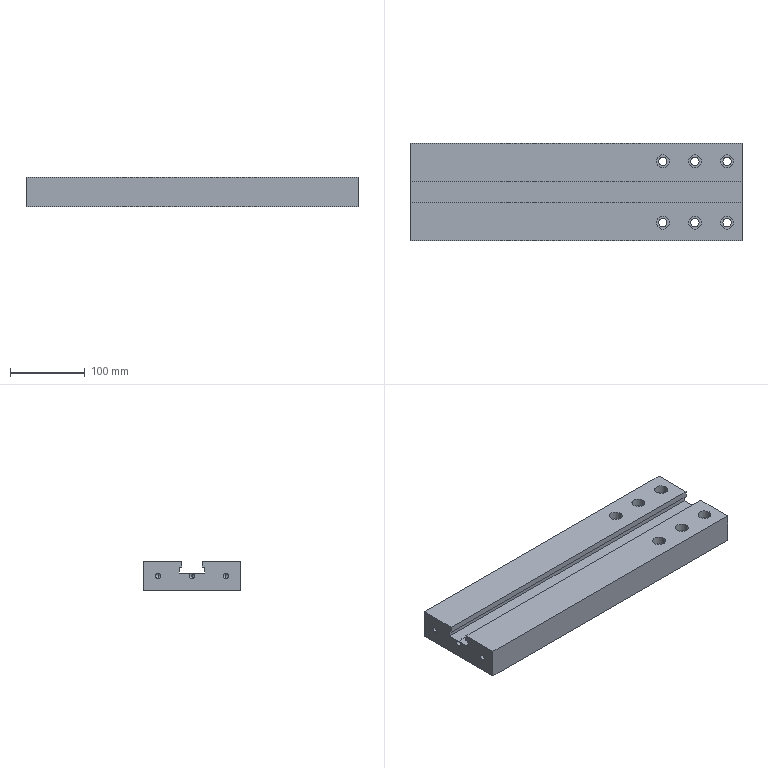Part | Creo | 1 solid | 59 faces | box 444 x 130 x 40 mm | volume 2055527 mm3 | cylinder 30 | plane 23 | cone 6 | commonest cylinder face diameters 11 x12 17.25 x12 6.985 x6